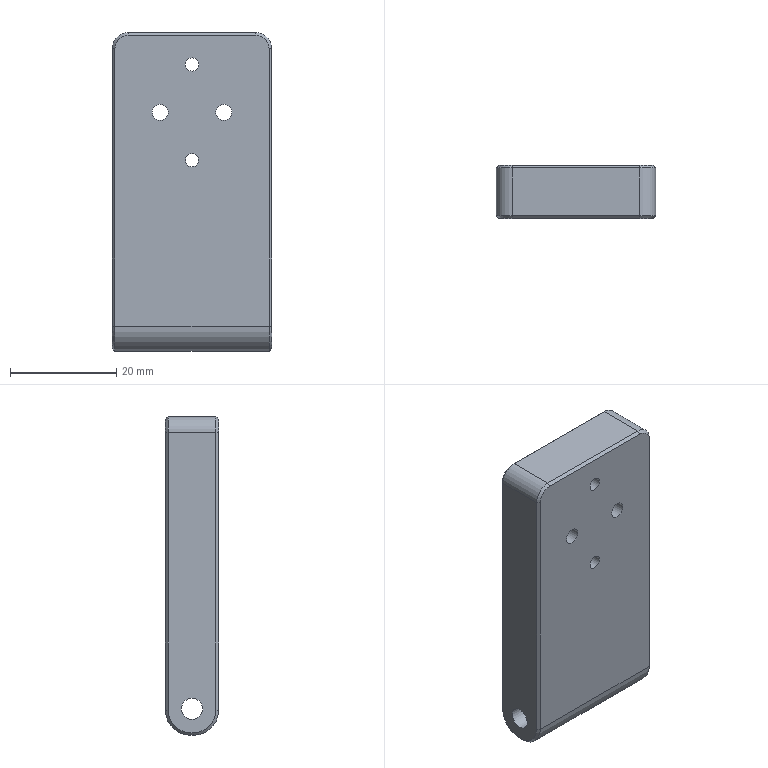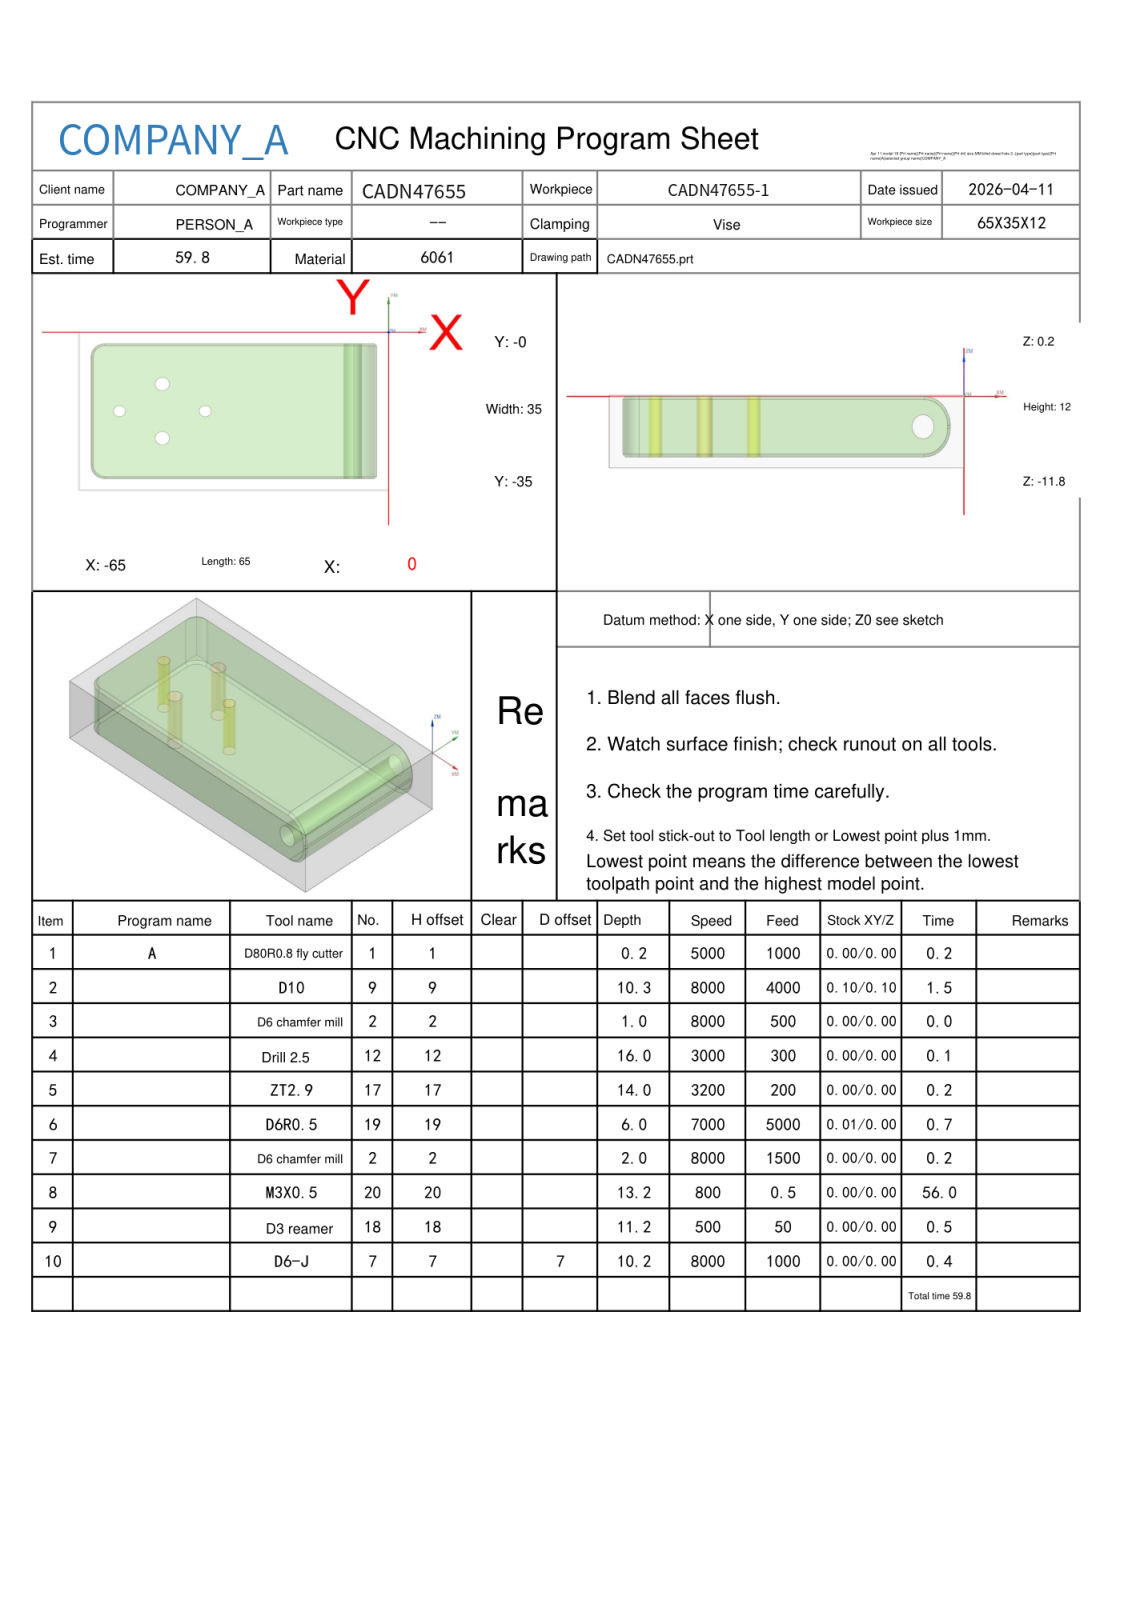NC program | NX | posted by the shop | part box 30 x 10 x 60 mm
Whole program:
%
O0001
(Machine time: 113.76 MIN)
(===Total Tool:9===)
(T1=D80R0.8 fly cutter D=80.  R=0.8  D-  H01 Z=0.    )
(T9=D10     D=10.  R=0.   D-  H09 Z=-10.1 )
(T2=D6 chamfer mill   D=6.   R=0.   D-  H02 Z=-1.8  )
(T12=Drill 2.5  D=2.5  DR_a=118 D-  H12 Z=-15.75)
(T17=ZT2.9  D=2.9  DR_a=120 D-  H17 Z=-13.84)
(T19=D6R0.5 D=6.   R=0.5  D-  H19 Z=-5.75 )
(T20=M3X0.5 D=2.5  DR_a=180 D-  H20 Z=-13.  )
(T18=D3 reamer   D=3.   DR_a=180 D-  H18 Z=-11.  )
(T7=D6-J    D=6.   R=0.   D7  H07 Z=-10.  )
G80 G90 G17 G49 G40
G91 G28 Z0
M01
N1 T01 M06
(D80R0.8 fly cutter  D=80. R=0.8 H=01 ce=0.00 di=0.00)
G00 G90 G54 X-107.5 Y-17.5 M03 S5000
G43 H01 Z20.
M08
Z2.
G01 Z0.0 F1000.
X-102.5
X37.5
X42.5
Z2.
G00 Z20.
G91 G28 Z0.0
M05
M09
G91 G28 Z0.0
M01
N2 T09 M06
(D10  D=10. R=0. H=09 ce=0.10 di=0.10)
G00 G90 G54 X-26.374 Y-47. M03 S8000
G43 H09 Z10.2
M08
Z.761
G01 Z-.439 F4000.
Y-45.979
G03 X-33.374 Y-38.979 I-7. J0.0
G01 X-59.5
G02 X-68.979 Y-29.5 I0.0 J9.479
G01 Y-5.5
G02 X-59.5 Y3.979 I9.479 J0.0
G01 X-7.252
G02 X-2.338 Y2.84 I-.216 J-12.102
X1.372 Y-2.993 I-2.73 J-5.833
G01 Y-32.011
G02 X-2.422 Y-37.887 I-6.447 J0.0
X-7.277 Y-38.979 I-5.086 J11.266
G01 X-33.374
G02 X-33.831 Y-38.617 I0.0 J.47
G01 X-33.893 Y-38.351
G03 X-34.867 Y-37.579 I-.974 J-.228
G01 X-59.5
G02 X-67.579 Y-29.5 I0.0 J8.079
G01 Y-5.5
G02 X-59.5 Y2.579 I8.079 J0.0
G01 X-7.277
G02 X-2.931 Y1.572 I-.191 J-10.702
X-.028 Y-2.993 I-2.137 J-4.565
G01 Y-32.011
G02 X-2.998 Y-36.611 I-5.047 J0.0
X-7.277 Y-37.579 I-4.51 J9.989
G01 X-33.374
X-33.874
G03 X-40.874 Y-44.579 I0.0 J-7.
G01 Y-47.
Z.761
G00 Z3.
G01 X-25.485 F6000.
G00 Z.322
G01 Z-.878 F4000.
Y-46.
G03 X-32.485 Y-39. I-7. J0.0
G01 X-59.5
G02 X-69. Y-29.5 I0.0 J9.5
G01 Y-5.5
G02 X-59.5 Y4. I9.5 J0.0
G01 X-5.472
G02 X-1.822 Y2.954 I-.142 J-7.39
X2.071 Y-3. I-2.716 J-6.026
G01 Y-32.019
G02 X-1.822 Y-37.954 I-6.609 J.091
X-5.498 Y-39. I-3.79 J6.341
G01 X-32.485
G02 X-32.943 Y-38.637 I0.0 J.47
G01 X-33.005 Y-38.372
G03 X-33.978 Y-37.6 I-.974 J-.228
G01 X-59.5
G02 X-67.6 Y-29.5 I0.0 J8.1
G01 Y-5.5
G02 X-59.5 Y2.6 I8.1 J0.0
G01 X-5.499
G02 X-2.471 Y1.711 I-.115 J-5.99
X.671 Y-3. I-2.067 J-4.782
G01 Y-32.
G02 X-2.471 Y-36.711 I-5.209 J.071
X-5.498 Y-37.6 I-3.142 J5.097
G01 X-32.485
X-32.985
G03 X-39.985 Y-44.6 I0.0 J-7.
G01 Y-47.
Z.322
G00 Z2.561
G01 X-25.147 F6000.
G00 Z-.117
G01 Z-1.317 F4000.
Y-44.6
G03 X-32.147 Y-37.6 I-7. J0.0
G01 X-59.5
G02 X-67.6 Y-29.5 I0.0 J8.1
G01 Y-5.5
G02 X-59.5 Y2.6 I8.1 J0.0
G01 X-4.793
G02 X-.945 Y1.1 I-.162 J-6.102
X1.176 Y-3. I-2.947 J-4.123
G01 Y-32.
G02 X-.945 Y-36.1 I-5.068 J.023
X-4.793 Y-37.6 I-4.016 J4.616
G01 X-32.147
X-32.647
G03 X-39.647 Y-44.6 I0.0 J-7.
G01 Y-47.
Z-.117
G00 Z2.122
G01 X-25.147 F6000.
G00 Z-.557
G01 Z-1.757 F4000.
Y-44.6
G03 X-32.147 Y-37.6 I-7. J0.0
G01 X-59.5
G02 X-67.6 Y-29.5 I0.0 J8.1
G01 Y-5.5
G02 X-59.5 Y2.6 I8.1 J0.0
G01 X-4.234
G02 X-.945 Y1.414 I-.045 J-5.278
X1.566 Y-3. I-2.802 J-4.515
G01 Y-32.
G02 X-.945 Y-36.414 I-5.312 J.101
X-4.233 Y-37.6 I-3.326 J4.069
G01 X-32.147
X-32.647
G03 X-39.647 Y-44.6 I0.0 J-7.
G01 Y-47.
Z-.557
G00 Z1.683
G01 X-25.147 F6000.
G00 Z-.996
G01 Z-2.196 F4000.
Y-44.6
G03 X-32.147 Y-37.6 I-7. J0.0
G01 X-59.5
G02 X-67.6 Y-29.5 I0.0 J8.1
G01 Y-5.5
G02 X-59.5 Y2.6 I8.1 J0.0
G01 X-3.896
G02 X-.056 Y.979 I-.053 J-5.486
X1.873 Y-3. I-3.265 J-4.04
G01 Y-32.
G02 X-.056 Y-35.979 I-5.194 J.061
X-3.897 Y-37.6 I-3.911 J3.905
G01 X-32.147
X-32.647
G03 X-39.647 Y-44.6 I0.0 J-7.
G01 Y-47.
Z-.996
G00 Z1.243
G01 X-25.147 F6000.
G00 Z-1.435
G01 Z-2.635 F4000.
Y-44.6
G03 X-32.147 Y-37.6 I-7. J0.0
G01 X-59.5
G02 X-67.6 Y-29.5 I0.0 J8.1
G01 Y-5.5
G02 X-59.5 Y2.6 I8.1 J0.0
G01 X-3.564
G02 X-.056 Y1.213 I-.06 J-5.28
X2.114 Y-3. I-3.244 J-4.337
G01 Y-32.
G02 X-.056 Y-36.213 I-5.415 J.124
X-3.563 Y-37.6 I-3.571 J3.901
G01 X-32.147
X-32.647
G03 X-39.647 Y-44.6 I0.0 J-7.
G01 Y-47.
Z-1.435
G00 Z.804
G01 X-25.147 F6000.
G00 Z-1.874
G01 Z-3.074 F4000.
Y-44.6
G03 X-32.147 Y-37.6 I-7. J0.0
G01 X-59.5
G02 X-67.6 Y-29.5 I0.0 J8.1
G01 Y-5.5
G02 X-59.5 Y2.6 I8.1 J0.0
G01 X-3.345
G02 X.576 Y.817 I-.097 J-5.418
X2.301 Y-3. I-3.456 J-3.86
G01 Y-32.
G02 X.576 Y-35.817 I-5.182 J.043
X-3.345 Y-37.6 I-4.018 J3.634
G01 X-32.147
X-32.647
G03 X-39.647 Y-44.6 I0.0 J-7.
G01 Y-47.
Z-1.874
G00 Z.365
G01 X-25.147 F6000.
G00 Z-2.313
G01 Z-3.513 F4000.
Y-44.6
G03 X-32.147 Y-37.6 I-7. J0.0
G01 X-59.5
G02 X-67.6 Y-29.5 I0.0 J8.1
G01 Y-5.5
G02 X-59.5 Y2.6 I8.1 J0.0
G01 X-3.261
X-3.24
G02 X.701 Y.817 I0.0 J-5.247
X2.44 Y-3. I-3.322 J-3.818
G01 Y-32.
G02 X.701 Y-35.817 I-5.06 J.001
X-3.255 Y-37.6 I-3.956 J3.497
G01 X-3.262
X-32.147
X-32.647
G03 X-39.647 Y-44.6 I0.0 J-7.
G01 Y-47.
Z-2.313
G00 Z-.074
G01 X-25.147 F6000.
G00 Z-2.752
G01 Z-3.952 F4000.
Y-44.6
G03 X-32.147 Y-37.6 I-7. J0.0
G01 X-59.5
G02 X-67.6 Y-29.5 I0.0 J8.1
G01 Y-5.5
G02 X-59.5 Y2.6 I8.1 J0.0
G01 X-3.075
G02 X.558 Y1.054 I-.05 J-5.159
X2.534 Y-3. I-3.379 J-4.156
G01 Y-32.
G02 X.812 Y-35.817 I-5.253 J.073
X-3.075 Y-37.6 I-3.998 J3.588
G01 X-32.147
X-32.647
G03 X-39.647 Y-44.6 I0.0 J-7.
G01 Y-47.
Z-2.752
G00 Z-.513
G01 X-25.147 F6000.
G00 Z-3.191
G01 Z-4.391 F4000.
Y-44.6
G03 X-32.147 Y-37.6 I-7. J0.0
G01 X-59.5
G02 X-67.6 Y-29.5 I0.0 J8.1
G01 Y-5.5
G02 X-59.5 Y2.6 I8.1 J0.0
G01 X-3.015
G02 X.833 Y.849 I-.081 J-5.284
X2.587 Y-3. I-3.579 J-3.955
G01 Y-32.
G02 X.833 Y-35.849 I-5.332 J.105
X-3.015 Y-37.6 I-3.933 J3.542
G01 X-32.147
X-32.647
G03 X-39.647 Y-44.6 I0.0 J-7.
G01 Y-47.
Z-3.191
G00 Z-.952
G01 X-25.147 F6000.
G00 Z-3.63
G01 Z-4.83 F4000.
Y-44.6
G03 X-32.147 Y-37.6 I-7. J0.0
G01 X-59.5
G02 X-67.6 Y-29.5 I0.0 J8.1
G01 Y-5.5
G02 X-59.5 Y2.6 I8.1 J0.0
G01 X-3.015
X-3.
G02 X.606 Y1.106 I0.0 J-5.1
G01 X1.106 Y.606
G02 X2.6 Y-3. I-3.606 J-3.606
G01 Y-32.
G02 X1.106 Y-35.606 I-5.1 J0.0
G01 X.606 Y-36.106
G02 X-3. Y-37.6 I-3.606 J3.606
G01 X-32.147
X-32.647
G03 X-39.647 Y-44.6 I0.0 J-7.
G01 Y-47.
Z-3.63
G00 Z-1.391
G01 X-25.147 F6000.
G00 Z-4.07
G01 Z-5.27 F4000.
Y-44.6
G03 X-32.147 Y-37.6 I-7. J0.0
G01 X-59.5
G02 X-67.6 Y-29.5 I0.0 J8.1
G01 Y-5.5
G02 X-59.5 Y2.6 I8.1 J0.0
G01 X-3.
G02 X.606 Y1.106 I0.0 J-5.1
G01 X1.106 Y.606
G02 X2.6 Y-3. I-3.606 J-3.606
G01 Y-32.
G02 X1.106 Y-35.606 I-5.1 J0.0
G01 X.606 Y-36.106
G02 X-3. Y-37.6 I-3.606 J3.606
G01 X-32.147
X-32.647
G03 X-39.647 Y-44.6 I0.0 J-7.
G01 Y-47.
Z-4.07
G00 Z-1.83
G01 X-25.147 F6000.
G00 Z-4.509
G01 Z-5.709 F4000.
Y-44.6
G03 X-32.147 Y-37.6 I-7. J0.0
G01 X-59.5
G02 X-67.6 Y-29.5 I0.0 J8.1
G01 Y-5.5
G02 X-59.5 Y2.6 I8.1 J0.0
G01 X-3.
G02 X.606 Y1.106 I0.0 J-5.1
G01 X1.106 Y.606
G02 X2.6 Y-3. I-3.606 J-3.606
G01 Y-32.
G02 X1.106 Y-35.606 I-5.1 J0.0
G01 X.606 Y-36.106
G02 X-3. Y-37.6 I-3.606 J3.606
G01 X-32.147
X-32.647
G03 X-39.647 Y-44.6 I0.0 J-7.
G01 Y-47.
Z-4.509
G00 Z-2.27
G01 X-25.147 F6000.
G00 Z-4.948
G01 Z-6.148 F4000.
Y-44.6
G03 X-32.147 Y-37.6 I-7. J0.0
G01 X-59.5
G02 X-67.6 Y-29.5 I0.0 J8.1
G01 Y-5.5
G02 X-59.5 Y2.6 I8.1 J0.0
G01 X-3.
G02 X.606 Y1.106 I0.0 J-5.1
G01 X1.106 Y.606
G02 X2.6 Y-3. I-3.606 J-3.606
G01 Y-32.
G02 X1.106 Y-35.606 I-5.1 J0.0
G01 X.606 Y-36.106
G02 X-3. Y-37.6 I-3.606 J3.606
G01 X-32.147
X-32.647
G03 X-39.647 Y-44.6 I0.0 J-7.
G01 Y-47.
Z-4.948
G00 Z-2.709
G01 X-25.147 F6000.
G00 Z-5.387
G01 Z-6.587 F4000.
Y-44.6
G03 X-32.147 Y-37.6 I-7. J0.0
G01 X-59.5
G02 X-67.6 Y-29.5 I0.0 J8.1
G01 Y-5.5
G02 X-59.5 Y2.6 I8.1 J0.0
G01 X-3.
G02 X.606 Y1.106 I0.0 J-5.1
G01 X1.106 Y.606
G02 X2.6 Y-3. I-3.606 J-3.606
G01 Y-32.
G02 X1.106 Y-35.606 I-5.1 J0.0
G01 X.606 Y-36.106
G02 X-3. Y-37.6 I-3.606 J3.606
G01 X-32.147
X-32.647
G03 X-39.647 Y-44.6 I0.0 J-7.
G01 Y-47.
Z-5.387
G00 Z-3.148
G01 X-25.147 F6000.
G00 Z-5.826
G01 Z-7.026 F4000.
Y-44.6
G03 X-32.147 Y-37.6 I-7. J0.0
G01 X-59.5
G02 X-67.6 Y-29.5 I0.0 J8.1
G01 Y-5.5
G02 X-59.5 Y2.6 I8.1 J0.0
G01 X-3.
G02 X.606 Y1.106 I0.0 J-5.1
G01 X1.106 Y.606
G02 X2.6 Y-3. I-3.606 J-3.606
G01 Y-32.
G02 X1.106 Y-35.606 I-5.1 J0.0
G01 X.606 Y-36.106
G02 X-3. Y-37.6 I-3.606 J3.606
G01 X-32.147
X-32.647
G03 X-39.647 Y-44.6 I0.0 J-7.
G01 Y-47.
Z-5.826
G00 Z-3.587
G01 X-25.147 F6000.
G00 Z-6.265
G01 Z-7.465 F4000.
Y-44.6
G03 X-32.147 Y-37.6 I-7. J0.0
G01 X-59.5
G02 X-67.6 Y-29.5 I0.0 J8.1
G01 Y-5.5
G02 X-59.5 Y2.6 I8.1 J0.0
G01 X-3.
G02 X.606 Y1.106 I0.0 J-5.1
G01 X1.106 Y.606
G02 X2.6 Y-3. I-3.606 J-3.606
G01 Y-32.
G02 X1.106 Y-35.606 I-5.1 J0.0
G01 X.606 Y-36.106
G02 X-3. Y-37.6 I-3.606 J3.606
G01 X-32.147
X-32.647
G03 X-39.647 Y-44.6 I0.0 J-7.
G01 Y-47.
Z-6.265
G00 Z-4.026
G01 X-25.147 F6000.
G00 Z-6.704
G01 Z-7.904 F4000.
Y-44.6
G03 X-32.147 Y-37.6 I-7. J0.0
G01 X-59.5
G02 X-67.6 Y-29.5 I0.0 J8.1
G01 Y-5.5
G02 X-59.5 Y2.6 I8.1 J0.0
G01 X-3.
G02 X.606 Y1.106 I0.0 J-5.1
G01 X1.106 Y.606
G02 X2.6 Y-3. I-3.606 J-3.606
G01 Y-32.
G02 X1.106 Y-35.606 I-5.1 J0.0
G01 X.606 Y-36.106
G02 X-3. Y-37.6 I-3.606 J3.606
G01 X-32.147
X-32.647
G03 X-39.647 Y-44.6 I0.0 J-7.
G01 Y-47.
Z-6.704
G00 Z-4.465
G01 X-25.147 F6000.
G00 Z-7.143
G01 Z-8.343 F4000.
Y-44.6
G03 X-32.147 Y-37.6 I-7. J0.0
G01 X-59.5
G02 X-67.6 Y-29.5 I0.0 J8.1
G01 Y-5.5
G02 X-59.5 Y2.6 I8.1 J0.0
G01 X-3.
G02 X.606 Y1.106 I0.0 J-5.1
G01 X1.106 Y.606
G02 X2.6 Y-3. I-3.606 J-3.606
G01 Y-32.
G02 X1.106 Y-35.606 I-5.1 J0.0
G01 X.606 Y-36.106
G02 X-3. Y-37.6 I-3.606 J3.606
G01 X-32.147
X-32.647
G03 X-39.647 Y-44.6 I0.0 J-7.
G01 Y-47.
Z-7.143
G00 Z-4.904
G01 X-25.147 F6000.
G00 Z-7.583
G01 Z-8.783 F4000.
Y-44.6
G03 X-32.147 Y-37.6 I-7. J0.0
G01 X-59.5
G02 X-67.6 Y-29.5 I0.0 J8.1
G01 Y-5.5
G02 X-59.5 Y2.6 I8.1 J0.0
G01 X-3.
G02 X.606 Y1.106 I0.0 J-5.1
G01 X1.106 Y.606
G02 X2.6 Y-3. I-3.606 J-3.606
G01 Y-32.
G02 X1.106 Y-35.606 I-5.1 J0.0
G01 X.606 Y-36.106
G02 X-3. Y-37.6 I-3.606 J3.606
G01 X-32.147
X-32.647
G03 X-39.647 Y-44.6 I0.0 J-7.
G01 Y-47.
Z-7.583
G00 Z-5.343
G01 X-25.147 F6000.
G00 Z-8.022
G01 Z-9.222 F4000.
Y-44.6
G03 X-32.147 Y-37.6 I-7. J0.0
G01 X-59.5
G02 X-67.6 Y-29.5 I0.0 J8.1
G01 Y-5.5
G02 X-59.5 Y2.6 I8.1 J0.0
G01 X-3.
G02 X.606 Y1.106 I0.0 J-5.1
G01 X1.106 Y.606
G02 X2.6 Y-3. I-3.606 J-3.606
G01 Y-32.
G02 X1.106 Y-35.606 I-5.1 J0.0
G01 X.606 Y-36.106
G02 X-3. Y-37.6 I-3.606 J3.606
G01 X-32.147
X-32.647
G03 X-39.647 Y-44.6 I0.0 J-7.
G01 Y-47.
Z-8.022
G00 Z-5.783
G01 X-25.147 F6000.
G00 Z-8.461
G01 Z-9.661 F4000.
Y-44.6
G03 X-32.147 Y-37.6 I-7. J0.0
G01 X-59.5
G02 X-67.6 Y-29.5 I0.0 J8.1
G01 Y-5.5
G02 X-59.5 Y2.6 I8.1 J0.0
G01 X-3.
G02 X.606 Y1.106 I0.0 J-5.1
G01 X1.106 Y.606
G02 X2.6 Y-3. I-3.606 J-3.606
G01 Y-32.
G02 X1.106 Y-35.606 I-5.1 J0.0
G01 X.606 Y-36.106
G02 X-3. Y-37.6 I-3.606 J3.606
G01 X-32.147
X-32.647
G03 X-39.647 Y-44.6 I0.0 J-7.
G01 Y-47.
Z-8.461
G00 Z-6.222
G01 X-25.147 F6000.
G00 Z-8.9
G01 Z-10.1 F4000.
Y-44.6
G03 X-32.147 Y-37.6 I-7. J0.0
G01 X-59.5
G02 X-67.6 Y-29.5 I0.0 J8.1
G01 Y-5.5
G02 X-59.5 Y2.6 I8.1 J0.0
G01 X-3.
G02 X.606 Y1.106 I0.0 J-5.1
G01 X1.106 Y.606
G02 X2.6 Y-3. I-3.606 J-3.606
G01 Y-32.
G02 X1.106 Y-35.606 I-5.1 J0.0
G01 X.606 Y-36.106
G02 X-3. Y-37.6 I-3.606 J3.606
G01 X-32.147
X-32.647
G03 X-39.647 Y-44.6 I0.0 J-7.
G01 Y-47.
Z-8.9
G00 Z10.2
G91 G28 Z0.0
M05
M09
G91 G28 Z0.0
M01
N3 T02 M06
(D6 chamfer mill  D=6. R=0. H=02 ce=0.00 di=0.10)
G00 G90 G54 X-38.5 Y-17.5 M03 S8000
G43 H02 Z20.
M08
G98 G81 X-38.5 Y-17.5 Z-.8 R1. F500.
X-47.5 Y-23.5
X-56.5 Y-17.5
X-47.5 Y-11.5
G80
G00 Z20.
G91 G28 Z0.0
M05
M09
G91 G28 Z0.0
M01
N4 T12 M06
(Drill 2.5 D=2.5 DR_a=118 H=12)
G00 G90 G54 X-56.5 Y-17.5 M03 S3000
G43 H12 Z20.
M08
G98 G83 X-56.5 Y-17.5 Z-15.751 R1. F300. Q2.
X-38.5
G80
G00 Z20.
G91 G28 Z0.0
M05
M09
G91 G28 Z0.0
M01
N5 T17 M06
(ZT2.9 D=2.9 DR_a=120 H=17)
G00 G90 G54 X-47.5 Y-23.5 M03 S3200
G43 H17 Z20.
M08
G98 G83 X-47.5 Y-23.5 Z-13.837 R1. F200. Q2.
Y-11.5
G80
G00 Z20.
G91 G28 Z0.0
M05
M09
G91 G28 Z0.0
M01
N6 T19 M06
(D6R0.5  D=6. R=0.5 H=19 ce=0.01 di=0.00)
G00 G90 G54 X-11.282 Y2.588 M03 S7000
G43 H19 Z10.2
M08
Z.494
G01 Z-.006 F5000.
Y2.576
G03 X-8.35 Y-.423 I3. J0.0
G02 X-7.836 Y-.406 I.514 J-7.698
X-6.275 Y-.566 I0.0 J-7.715
X-4.486 Y-3. I-.989 J-2.602
G01 Y-32.
G02 X-6.646 Y-34.492 I-2.617 J.086
X-7.832 Y-34.597 I-1.186 J6.688
X-8.35 Y-34.577 I0.0 J6.792
G01 X-8.463 Y-34.622 Z-.013
X-8.349 Y-34.623
X-6.966 Y-34.611
X-6.902 Y-34.605
G03 X-4.367 Y-32. I-.197 J2.728
G01 Y-3.
G03 X-6.902 Y-.395 I-2.734 J-.124
G01 X-6.966 Y-.389
X-8.349 Y-.377
X-8.463 Y-.378
X-8.437 Y-.347 Z-.022
X-6.966 Y-.358
G02 X-4.255 Y-3. I-.039 J-2.753
G01 Y-32.
G02 X-6.713 Y-34.617 I-2.722 J.094
G01 X-6.966 Y-34.642
X-8.437 Y-34.653
X-8.409 Y-34.689 Z-.034
G03 X-7.868 Y-34.703 I.541 J10.769
X-6.551 Y-34.622 I0.0 J10.782
X-4.147 Y-32. I-.335 J2.72
G01 Y-3.
G03 X-6.551 Y-.378 I-2.739 J-.098
X-7.868 Y-.297 I-1.317 J-10.702
X-8.409 Y-.311 I0.0 J-10.782
G01 X-8.388 Y-.284 Z-.047
X-6.966 Y-.291
X-6.62 Y-.323
G02 X-4.042 Y-3. I-.247 J-2.818
G01 Y-32.
G02 X-6.62 Y-34.677 I-2.826 J.142
G01 X-6.966 Y-34.709
X-8.388 Y-34.716
X-8.364 Y-34.747 Z-.062
G03 X-7.783 Y-34.764 I.581 J10.111
X-6.275 Y-34.651 I0.0 J10.127
X-3.939 Y-32. I-.436 J2.739
G01 Y-3.
G03 X-6.275 Y-.349 I-2.772 J-.088
X-7.783 Y-.236 I-1.508 J-10.014
X-8.364 Y-.253 I0.0 J-10.127
G01 X-8.408 Y-.226 Z-.078
G02 X-7.802 Y-.211 I.606 J-11.862
X-6.275 Y-.309 I0.0 J-11.878
X-3.837 Y-3. I-.397 J-2.81
G01 Y-32.
G02 X-6.275 Y-34.691 I-2.835 J.119
X-7.802 Y-34.789 I-1.527 J11.779
X-8.408 Y-34.774 I0.0 J11.878
G01 X-8.387 Y-34.8 Z-.097
X-6.966 Y-34.794
G03 X-5.154 Y-34.336 I-.065 J4.072
X-3.735 Y-32. I-1.213 J2.336
G01 Y-2.948
G03 X-4.214 Y-1.51 I-2.397 J0.0
X-6.62 Y-.227 I-2.574 J-1.93
G01 X-6.966 Y-.206
X-8.387 Y-.2
X-8.364 Y-.171 Z-.118
X-6.966 Y-.184
X-6.62 Y-.203
G02 X-4.191 Y-1.395 I-.111 J-3.299
X-3.635 Y-2.935 I-1.856 J-1.54
G01 Y-32.
G02 X-5.238 Y-34.443 I-2.75 J.056
G01 X-5.432 Y-34.521
G02 X-6.946 Y-34.816 I-1.536 J3.843
G01 X-8.343 Y-34.824
X-8.364 Y-34.829
X-8.361 Y-34.845 Z-.129
X-8.359 Y-34.856 Z-.14
X-6.966 Y-34.841
X-6.955
G03 X-5.238 Y-34.49 I0.0 J4.381
X-3.536 Y-32. I-1.051 J2.545
G01 Y-3.
G03 X-3.855 Y-1.751 I-2.997 J-.1
X-6.275 Y-.214 I-2.728 J-1.621
X-8.051 Y-.142 I-1.776 J-21.903
X-8.359 Y-.144 I0.0 J-21.975
G01 X-8.36 Y-.119 Z-.164
G02 X-7.985 Y-.115 I.375 J-19.937
X-6.275 Y-.189 I0.0 J-19.941
X-3.757 Y-1.761 I-.228 J-3.166
X-3.437 Y-2.949 I-2.047 J-1.189
G01 Y-32.001
G02 X-4.865 Y-34.368 I-2.674 J0.0
X-6.62 Y-34.846 I-1.957 J3.716
G01 X-6.966 Y-34.867
X-8.36 Y-34.881
X-8.351 Y-34.907 Z-.19
G03 X-8.007 Y-34.91 I.343 J27.25
X-6.62 Y-34.874 I0.0 J27.253
X-4.892 Y-34.443 I-.196 J4.465
X-3.339 Y-32. I-1.218 J2.489
G01 Y-3.
G03 X-4.56 Y-.754 I-2.677 J0.0
X-6.275 Y-.161 I-2.055 J-3.169
X-7.895 Y-.087 I-1.62 J-17.514
X-8.351 Y-.093 I0.0 J-17.589
G01 X-8.349 Y-.065 Z-.218
G02 X-7.809 Y-.054 I.54 J-13.475
X-5.929 Y-.186 I0.0 J-13.486
X-3.779 Y-1.408 I-.419 J-3.24
X-3.242 Y-2.962 I-1.979 J-1.554
G01 Y-32.
G02 X-4.892 Y-34.492 I-2.788 J.054
X-6.62 Y-34.904 I-1.964 J4.404
X-7.901 Y-34.94 I-1.281 J22.988
X-8.349 Y-34.935 I0.0 J23.023
G01 Y-34.965 Z-.248
X-6.851 Y-34.951
X-6.62 Y-34.936
G03 X-4.892 Y-34.544 I-.3 J5.335
X-3.146 Y-32. I-1.068 J2.605
G01 Y-2.967
G03 X-3.69 Y-1.397 I-2.535 J0.0
X-5.737 Y-.187 I-2.588 J-2.041
X-7.756 Y-.021 I-2.018 J-12.143
X-8.349 Y-.035 I0.0 J-12.31
G01 Y-.003 Z-.28
G02 X-7.811 Y.004 I.538 J-19.763
X-6.62 Y-.032 I0.0 J-19.771
X-4.892 Y-.4 I-.472 J-6.451
X-3.05 Y-3. I-1.002 J-2.663
G01 Y-32.
G02 X-4.892 Y-34.6 I-2.844 J.063
X-6.966 Y-34.989 I-2.266 J6.353
G01 X-8.349 Y-34.997
Y-35.03 Z-.313
X-7.166 Y-35.023
G03 X-4.884 Y-34.636 I-.041 J7.161
X-2.955 Y-32. I-.927 J2.703
G01 Y-3.
G03 X-4.883 Y-.365 I-2.856 J-.067
X-6.85 Y.014 I-2.317 J-6.745
X-7.812 Y.037 I-.962 J-19.601
X-8.349 Y.03 I0.0 J-19.625
G01 Y.065 Z-.348
G02 X-7.813 Y.073 I.535 J-19.466
X-6.62 Y.036 I0.0 J-19.473
X-4.546 Y-.461 I-.467 J-6.522
X-2.86 Y-3. I-1.152 J-2.594
G01 Y-32.
G02 X-4.546 Y-34.539 I-2.838 J.055
X-7.091 Y-35.058 I-2.585 J6.179
G01 X-8.349 Y-35.065
Y-35.102 Z-.385
X-7.312
X-7.279
G03 X-4.546 Y-34.594 I0.0 J7.605
X-2.767 Y-32. I-1.094 J2.659
G01 Y-3.
G03 X-4.546 Y-.406 I-2.874 J-.064
X-7.163 Y.095 I-2.663 J-6.835
G01 X-8.349 Y.102
Y.141 Z-.424
X-7.236 Y.133
G02 X-4.523 Y-.373 I-.051 J-7.788
X-2.674 Y-3. I-1.018 J-2.681
G01 Y-32.
G02 X-4.546 Y-34.635 I-2.867 J.054
X-7.294 Y-35.141 I-2.748 J7.216
G01 X-7.312
X-8.349
Y-35.181 Z-.464
X-7.312
X-7.304
G03 X-4.546 Y-34.674 I0.0 J7.75
G01 X-4.361 Y-34.605
G03 X-2.582 Y-32. I-1.113 J2.67
G01 Y-3.
G03 X-4.361 Y-.395 I-2.892 J-.065
G01 X-4.546 Y-.326
G03 X-7.182 Y.173 I-2.687 J-6.983
G01 X-8.349 Y.181
Y.223 Z-.506
G02 X-7.819 Y.231 I.53 J-18.812
X-6.823 Y.205 I0.0 J-18.82
X-4.228 Y-.408 I-.396 J-7.479
X-2.49 Y-3. I-1.156 J-2.654
G01 Y-32.
G02 X-4.201 Y-34.58 I-2.894 J.062
X-7.312 Y-35.223 I-3.129 J7.281
G01 X-8.349
Y-35.267 Z-.55
X-7.312
G03 X-4.201 Y-34.627 I-.047 J8.11
X-2.4 Y-32. I-1.101 J2.685
G01 Y-3.
G03 X-4.201 Y-.373 I-2.902 J-.058
X-6.62 Y.236 I-3.222 J-7.689
X-7.82 Y.275 I-1.2 J-18.608
X-8.349 Y.267 I0.0 J-18.646
G01 X-8.341 Y.313 Z-.596
X-6.966 Y.302
G02 X-3.855 Y-.497 I-.304 J-7.64
X-2.311 Y-3. I-1.321 J-2.543
G01 Y-32.
G02 X-3.855 Y-34.503 I-2.866 J.04
X-6.966 Y-35.302 I-3.416 J6.842
G01 X-8.341 Y-35.313
X-8.346 Y-35.36 Z-.643
G03 X-7.923 Y-35.364 I.423 J22.426
X-6.986 Y-35.345 I0.0 J22.43
X-3.852 Y-34.555 I-.332 J7.928
X-2.222 Y-32. I-1.264 J2.604
G01 Y-3.
G03 X-3.852 Y-.445 I-2.894 J-.049
X-6.988 Y.344 I-3.463 J-7.132
X-7.935 Y.364 I-.947 J-22.92
X-8.346 Y.36 I0.0 J-22.939
G01 X-8.341 Y.384 Z-.668
X-8.336 Y.409 Z-.692
G02 X-7.901 Y.414 I.435 J-17.169
X-6.275 Y.337 I0.0 J-17.175
X-3.845 Y-.395 I-1.327 J-8.806
X-2.135 Y-3. I-1.221 J-2.665
G01 Y-32.
G02 X-3.845 Y-34.605 I-2.931 J.06
X-6.62 Y-35.372 I-3.61 J7.658
X-7.917 Y-35.412 I-1.297 J21.012
X-8.336 Y-35.408 I0.0 J21.052
G01 X-8.335 Y-35.433 Z-.717
Y-35.458 Z-.743
X-7.312 Y-35.455
G03 X-3.509 Y-34.473 I-.061 J8.088
X-2.048 Y-32. I-1.428 J2.512
G01 Y-3.
G03 X-3.509 Y-.527 I-2.889 J-.04
X-7.312 Y.454 I-3.858 J-7.093
G01 X-8.334 Y.459
Y.485 Z-.769
X-8.333 Y.511 Z-.795
X-7.312 Y.504
G02 X-3.509 Y-.476 I-.069 J-8.137
X-1.962 Y-3. I-1.352 J-2.565
G01 Y-32.
G02 X-3.509 Y-34.524 I-2.899 J.041
X-7.312 Y-35.505 I-3.88 J7.18
G01 X-8.333 Y-35.51
X-8.332 Y-35.536 Z-.822
X-8.331 Y-35.563 Z-.849
G03 X-7.993 Y-35.565 I.337 J23.996
X-6.966 Y-35.543 I0.0 J23.998
X-3.257 Y-34.426 I-.399 J8.038
X-1.878 Y-32.003 I-1.438 J2.423
G01 Y-2.997
G03 X-3.257 Y-.574 I-2.817 J0.0
X-6.62 Y.517 I-4.1 J-6.907
X-8.034 Y.567 I-1.413 J-20.128
X-8.331 Y.565 I0.0 J-20.177
G01 X-8.329 Y.592 Z-.877
X-8.328 Y.62 Z-.904
G02 X-7.994 Y.624 I.335 J-15.944
X-6.275 Y.531 I0.0 J-15.947
X-3.164 Y-.566 I-1.239 J-8.478
X-1.794 Y-3. I-1.564 J-2.482
G01 Y-32.
G02 X-3.164 Y-34.434 I-2.934 J.048
X-7.312 Y-35.611 I-4.298 J7.251
G01 X-8.328 Y-35.618
X-8.327 Y-35.646 Z-.933
X-8.326 Y-35.674 Z-.961
X-7.312 Y-35.666
G03 X-3.164 Y-34.485 I-.169 J8.468
X-1.712 Y-32. I-1.464 J2.522
G01 Y-3.
G03 X-3.164 Y-.515 I-2.916 J-.038
X-6.275 Y.583 I-4.353 J-7.379
X-8.011 Y.68 I-1.737 J-15.455
X-8.326 Y.677 I0.0 J-15.552
G01 X-8.325 Y.706 Z-.991
X-8.324 Y.735 Z-1.02
G02 X-8.01 Y.738 I.314 J-14.775
X-6.678 Y.678 I0.0 J-14.778
X-2.919 Y-.622 I-.746 J-8.24
X-1.63 Y-2.995 I-1.54 J-2.373
G01 Y-32.001
G02 X-2.934 Y-34.387 I-2.836 J0.0
X-7.312 Y-35.722 I-4.555 J7.093
G01 X-8.324 Y-35.732
X-8.323 Y-35.762 Z-1.05
X-8.322 Y-35.792 Z-1.08
G03 X-8.062 Y-35.794 I.26 J18.062
X-7.015 Y-35.763 I0.0 J18.064
X-2.818 Y-34.373 I-.495 J8.522
X-1.55 Y-32. I-1.656 J2.41
G01 Y-3.
G03 X-2.818 Y-.627 I-2.923 J-.037
X-6.774 Y.745 I-4.685 J-7.118
X-8.015 Y.798 I-1.241 J-14.453
X-8.322 Y.795 I0.0 J-14.506
G01 X-8.321 Y.826 Z-1.111
X-8.32 Y.856 Z-1.142
G02 X-8.091 Y.858 I.229 J-17.323
X-7.016 Y.824 I0.0 J-17.324
X-3.107 Y-.395 I-.534 J-8.591
G01 X-2.818 Y-.565
G02 X-1.471 Y-3. I-1.607 J-2.479
G01 Y-32.
G02 X-2.818 Y-34.435 I-2.957 J.045
G01 X-3.186 Y-34.652
G02 X-7.04 Y-35.824 I-4.34 J7.352
X-8.109 Y-35.854 I-1.07 J18.757
X-8.32 Y-35.853 I0.0 J18.788
G01 X-8.319 Y-35.884 Z-1.173
X-8.317 Y-35.915 Z-1.205
X-8.165 Y-35.916
G03 X-7.064 Y-35.885 I0.0 J19.675
X-3.213 Y-34.717 I-.476 J8.499
G01 X-2.818 Y-34.483
G03 X-1.393 Y-32. I-1.514 J2.519
G01 Y-2.999
G03 X-2.642 Y-.639 I-2.855 J0.0
X-6.275 Y.813 I-5.099 J-7.49
X-8.029 Y.922 I-1.755 J-14.038
X-8.317 Y.919 I0.0 J-14.147
G01 X-8.316 Y.951 Z-1.237
X-8.315 Y.983 Z-1.269
G02 X-8.037 Y.986 I.278 J-13.963
X-6.275 Y.874 I0.0 J-13.966
X-2.543 Y-.651 I-1.543 J-9.1
X-1.317 Y-3. I-1.636 J-2.349
G01 Y-32.003
G02 X-2.538 Y-34.345 I-2.856 J0.0
X-6.275 Y-35.873 I-5.263 J7.538
X-8.06 Y-35.981 I-1.786 J14.652
X-8.315 Y-35.979 I0.0 J14.761
G01 X-8.154 Y-36.042 Z-1.335
X-7.971 Y-36.043
G03 X-6.275 Y-35.936 I0.0 J13.476
X-2.818 Y-34.583 I-1.546 J9.048
G01 X-2.472 Y-34.36
G03 X-1.242 Y-32. I-1.712 J2.394
G01 Y-3.
G03 X-2.472 Y-.64 I-2.943 J-.034
G01 X-2.818 Y-.417
G03 X-6.275 Y.937 I-5.03 J-7.752
X-7.918 Y1.049 I-1.643 J-12.099
X-8.143 Y1.046 I0.0 J-12.21
G01 X-8.024 Y1.068 Z-1.358
X-7.904 Y1.088 Z-1.38
X-7.784 Y1.108 Z-1.403
X-7.599 Y1.11
G02 X-4.736 Y.589 I0.0 J-8.123
G01 X-4.546 Y.517
G02 X-2.349 Y-.678 I-3.452 J-8.965
X-1.168 Y-2.998 I-1.687 J-2.32
G01 Y-32.002
G02 X-2.349 Y-34.322 I-2.868 J0.0
X-5.929 Y-35.939 I-5.687 J7.823
X-7.697 Y-36.101 I-1.768 J9.523
G01 X-7.839 Y-36.1
X-7.682 Y-36.109 Z-1.414
X-7.524 Y-36.117 Z-1.426
X-7.367 Y-36.125 Z-1.437
X-7.209 Y-36.132 Z-1.449
X-7.052 Y-36.133 Z-1.46
X-6.895 Y-36.132 Z-1.472
G03 X-5.238 Y-35.824 I-.404 J6.775
X-2.278 Y-34.328 I-3.116 J9.843
X-1.095 Y-32.004 I-1.691 J2.324
G01 Y-2.998
G03 X-2.272 Y-.676 I-2.879 J0.0
X-4.724 Y.642 I-5.922 J-8.08
X-6.835 Y1.135 I-2.66 J-6.618
G01 X-6.69 Y1.137 Z-1.486
X-6.545 Z-1.5
X-6.4 Y1.132 Z-1.514
X-6.257 Y1.12 Z-1.528
X-6.114 Y1.105 Z-1.542
G02 X-5.002 Y.806 I-.973 J-5.835
G01 X-4.733 Y.705
G02 X-2.108 Y-.74 I-3.708 J-9.845
X-1.023 Y-3. I-1.881 J-2.292
G01 Y-32.
G02 X-2.108 Y-34.26 I-2.965 J.033
X-5.238 Y-35.889 I-6.488 J8.641
X-6.123 Y-36.105 I-1.808 J5.502
G01 X-5.952 Y-36.099 Z-1.566
X-5.781 Y-36.088 Z-1.59
X-5.614 Y-36.064 Z-1.614
G03 X-2.127 Y-34.325 I-2.92 J10.224
X-.953 Y-32. I-1.761 J2.347
G01 Y-3.
G03 X-2.127 Y-.675 I-2.934 J-.022
X-5.613 Y1.064 I-6.428 J-8.522
G01 X-5.487 Y1.052 Z-1.638
X-5.362 Y1.038 Z-1.662
X-5.236 Y1.024 Z-1.686
G02 X-2.022 Y-.699 I-3.738 J-10.831
X-.885 Y-2.999 I-1.755 J-2.299
G01 Y-32.001
G02 X-2.022 Y-34.301 I-2.893 J0.0
X-5.235 Y-36.024 I-6.955 J9.112
G01 X-5.082 Y-36.01 Z-1.723
X-4.932 Y-35.986 Z-1.761
G03 X-2.127 Y-34.43 I-4.357 J11.167
G01 X-1.898 Y-34.26
G03 X-.817 Y-32. I-1.889 J2.291
G01 Y-3.
G03 X-1.898 Y-.74 I-2.969 J-.031
G01 X-2.127 Y-.57
G03 X-4.933 Y.985 I-7.158 J-9.607
G01 X-4.804 Y.968 Z-1.798
X-4.676 Y.949 Z-1.836
G02 X-1.781 Y-.779 I-4.92 J-11.535
X-.752 Y-3. I-1.948 J-2.252
G01 Y-32.
G02 X-1.781 Y-34.221 I-2.977 J.03
X-4.675 Y-35.949 I-7.825 J9.821
G01 X-4.557 Y-35.936 Z-1.874
X-4.443 Y-35.915 Z-1.913
G03 X-1.814 Y-34.305 I-5.913 J12.606
X-.687 Y-32.004 I-1.788 J2.301
G01 Y-2.996
G03 X-1.814 Y-.695 I-2.914 J0.0
X-4.444 Y.915 I-8.53 J-10.979
G01 X-4.339 Y.902 Z-1.952
X-4.237 Y.882 Z-1.991
G02 X-1.691 Y-.74 I-6.428 J-12.895
X-.624 Y-3. I-1.892 J-2.275
G01 Y-32.
G02 X-1.691 Y-34.26 I-2.959 J.015
X-4.236 Y-35.882 I-8.987 J11.289
G01 X-4.14 Y-35.868 Z-2.03
X-4.045 Y-35.849 Z-2.07
G03 X-1.673 Y-34.297 I-7.323 J13.784
X-.563 Y-32.001 I-1.82 J2.296
G01 Y-2.999
G03 X-1.673 Y-.703 I-2.93 J0.0
X-4.046 Y.849 I-9.681 J-12.215
G01 X-3.948 Y.837 Z-2.11
X-3.855 Y.819 Z-2.15
G02 X-2.471 Y-.049 I-18.846 J-31.574
G01 X-1.657 Y-.669
G02 X-.503 Y-2.997 I-1.771 J-2.328
G01 Y-32.003
G02 X-1.657 Y-34.331 I-2.926 J0.0
G01 X-2.471 Y-34.951
G02 X-3.854 Y-35.819 I-19.942 J30.235
G01 X-3.709 Y-35.788 Z-2.231
G03 X-2.928 Y-35.296 I-4.228 J7.582
X-1.435 Y-34.196 I-7.201 J11.33
X-.445 Y-32. I-1.96 J2.206
G01 Y-3.
G03 X-1.435 Y-.804 I-2.951 J-.009
X-2.928 Y.296 I-8.653 J-10.18
X-3.709 Y.788 I-5.02 J-7.107
G01 X-3.558 Y.764 Z-2.314
G02 X-1.435 Y-.747 I-10.232 J-16.617
X-.388 Y-3. I-1.933 J-2.268
G01 Y-32.
G02 X-1.435 Y-34.253 I-2.98 J.016
X-3.558 Y-35.764 I-12.332 J15.073
G01 X-3.422 Y-35.742 Z-2.397
G03 X-1.388 Y-34.26 I-11.283 J17.621
X-.333 Y-32. I-1.928 J2.276
G01 Y-3.
G03 X-1.388 Y-.74 I-2.982 J-.016
X-3.422 Y.742 I-12.952 J-15.643
G01 X-3.294 Y.717 Z-2.482
G02 X-1.332 Y-.74 I-11.6 J-17.664
X-.279 Y-3. I-1.927 J-2.273
G01 Y-32.
G02 X-1.332 Y-34.26 I-2.98 J.014
X-3.294 Y-35.718 I-13.609 J16.259
G01 X-3.164 Y-35.694 Z-2.567
X-2.607 Y-35.296
X-2.472 Y-35.196
X-2.258 Y-35.043
G03 X-1.435 Y-34.387 I-5.978 J8.345
G01 X-1.276 Y-34.26
G03 X-.227 Y-32. I-1.947 J2.277
G01 Y-2.996
G03 X-1.335 Y-.693 I-2.947 J0.0
G01 X-1.435 Y-.613
G03 X-2.26 Y.044 I-6.759 J-7.638
G01 X-2.472 Y.196
X-2.608 Y.296
X-3.165 Y.694
X-3.052 Y.671 Z-2.654
X-3.009 Y.642
X-2.127 Y-.008
X-2.063 Y-.049
G02 X-1.225 Y-.74 I-23.386 J-29.194
X-.177 Y-3. I-1.942 J-2.274
G01 Y-32.
G02 X-1.225 Y-34.26 I-2.991 J.015
X-2.063 Y-34.951 I-24.493 J28.825
G01 X-2.127 Y-34.993
X-3.008 Y-35.642
X-3.052 Y-35.672
X-2.937 Y-35.651 Z-2.741
X-2.004 Y-34.951
X-1.781 Y-34.774
X-1.176 Y-34.26
G03 X-.128 Y-32. I-1.941 J2.272
G01 Y-3.
G03 X-1.176 Y-.74 I-2.988 J-.013
G01 X-1.781 Y-.226
X-2.004 Y-.049
X-2.937 Y.65
X-2.835 Y.631 Z-2.829
X-1.781 Y-.183
X-1.126 Y-.74
G02 X-.081 Y-3. I-1.958 J-2.276
G01 Y-32.
G02 X-1.09 Y-34.226 I-2.991 J.013
G01 X-1.781 Y-34.817
X-1.949 Y-34.951
X-2.127 Y-35.082
X-2.834 Y-35.631
X-2.745 Y-35.616 Z-2.919
X-1.896 Y-34.951
X-1.781 Y-34.86
X-1.09 Y-34.27
G03 X-.036 Y-32. I-1.958 J2.288
G01 Y-3.
G03 X-1.09 Y-.73 I-3.013 J-.019
G01 X-1.781 Y-.14
X-2.746 Y.616
X-2.658 Y.601 Z-3.009
X-2.127 Y.172
X-1.841 Y-.049
G02 X-.903 Y-.868 I-8.475 J-10.66
X.007 Y-2.998 I-2.038 J-2.13
G01 Y-32.
G02 X-.744 Y-33.975 I-3.023 J.02
X-1.841 Y-34.951 I-9.093 J9.119
G01 X-2.127 Y-35.173
X-2.657 Y-35.601
X-2.569 Y-35.584 Z-3.099
X-2.472 Y-35.503
X-1.942 Y-35.076
G03 X-.744 Y-34.023 I-11.432 J14.205
X.049 Y-32. I-2.218 J2.037
G01 Y-2.998
G03 X-.877 Y-.851 I-2.951 J0.0
X-1.927 Y.064 I-12.076 J-12.804
G01 X-2.472 Y.502
X-2.57 Y.584
X-2.484 Y.564 Z-3.191
X-2.127 Y.265
X-1.781 Y-.016
G02 X-.856 Y-.829 I-13.816 J-16.663
X.089 Y-2.999 I-2.018 J-2.171
G01 Y-32.001
G02 X-.857 Y-34.172 I-2.964 J0.0
X-1.781 Y-34.984 I-14.868 J15.992
G01 X-2.127 Y-35.265
X-2.483 Y-35.564
X-2.414 Y-35.553 Z-3.284
G03 X-.744 Y-34.107 I-23.728 J29.093
X.128 Y-32. I-2.164 J2.129
G01 Y-3.
G03 X-.744 Y-.893 I-3.036 J-.023
X-2.415 Y.553 I-25.012 J-27.217
G01 X-2.348 Y.542 Z-3.377
X-1.781 Y.057
X-1.594 Y-.097
G02 X-.65 Y-.956 I-8.265 J-10.027
X.164 Y-3. I-2.2 J-2.061
G01 Y-32.
G02 X-.744 Y-34.144 I-3.038 J.023
G01 X-.872 Y-34.26
X-1.249 Y-34.605
G02 X-1.781 Y-35.058 I-5.654 J6.107
G01 X-2.348 Y-35.543
X-2.281 Y-35.533 Z-3.47
X-1.781 Y-35.095
X-1.606 Y-34.951
G03 X-.83 Y-34.26 I-11.455 J13.643
G01 X-.744 Y-34.178
G03 X.199 Y-32. I-2.11 J2.207
G01 Y-3.
G03 X-.57 Y-1. I-3.063 J-.029
X-1.606 Y-.049 I-10.338 J-10.237
G01 X-1.781 Y.095
X-2.281 Y.532
X-2.217 Y.517 Z-3.565
G02 X-1.781 Y.132 I-26.961 J-30.939
G01 X-1.435 Y-.156
G02 X-.576 Y-.956 I-15.73 J-17.762
X.232 Y-3. I-2.262 J-2.076
G01 Y-32.
G02 X-.576 Y-34.044 I-3.07 J.032
X-1.634 Y-35.01 I-11.465 J11.498
G01 X-1.781 Y-35.132
X-2.217 Y-35.518
X-2.153 Y-35.502 Z-3.66
G03 X-.672 Y-34.173 I-37.004 J42.736
X.263 Y-32. I-2.091 J2.189
G01 Y-3.
G03 X-.545 Y-.956 I-3.026 J-.016
X-1.781 Y.17 I-14.584 J-14.77
X-2.154 Y.501 I-157.33 J-176.326
G01 X-2.102 Y.494 Z-3.755
G02 X-.6 Y-.87 I-31.203 J-35.858
X.293 Y-3. I-2.126 J-2.143
G01 Y-32.
G02 X-.6 Y-34.13 I-3.017 J.013
X-2.101 Y-35.495 I-33.414 J35.249
G01 X-2.058 Y-35.493 Z-3.852
G03 X-.615 Y-34.173 I-50.87 J57.085
X.32 Y-32. I-2.086 J2.186
G01 Y-3.
G03 X-.615 Y-.827 I-3.023 J-.013
X-2.059 Y.493 I-49.787 J-53.041
G01 X-2.02 Y.487 Z-3.948
G02 X-.637 Y-.784 I-37.232 J-41.893
X.346 Y-3. I-2.018 J-2.222
G01 Y-32.
G02 X-.637 Y-34.216 I-3.001 J.005
X-2.019 Y-35.487 I-40.972 J43.154
G01 X-1.98 Y-35.48 Z-4.045
G03 X-.543 Y-34.149 I-32.011 J36.015
X.37 Y-32.001 I-2.072 J2.149
G01 Y-3.
G03 X-.52 Y-.87 I-3.018 J-.01
X-1.981 Y.48 I-34.974 J-36.385
G01 X-1.943 Y.473 Z-4.143
G02 X-.515 Y-.853 I-28.869 J-32.526
X.392 Y-2.998 I-2.083 J-2.145
G01 Y-32.
G02 X-.495 Y-34.13 I-3.034 J.014
X-1.942 Y-35.473 I-34.328 J35.514
G01 X-1.902 Y-35.467 Z-4.241
G03 X-1.435 Y-35.031 I-11.586 J12.886
X-.57 Y-34.216 I-8.24 J9.625
G01 X-.528 Y-34.173
X-.476 Y-34.13
G03 X.412 Y-32. I-2.137 J2.141
G01 Y-2.999
G03 X-.489 Y-.86 I-2.987 J0.0
G01 X-1.09 Y-.274
G02 X-1.904 Y.466 I21.759 J24.734
G01 X-1.867 Y.457 Z-4.339
G02 X-.5 Y-.827 I-51.156 J-55.857
X.43 Y-3. I-2.095 J-2.182
G01 Y-32.
G02 X-.456 Y-34.13 I-3.02 J.007
G01 X-.508 Y-34.173
X-.727 Y-34.392
G02 X-1.435 Y-35.051 I-9.627 J9.637
X-1.865 Y-35.457 I-17.372 J17.922
G01 X-1.829 Y-35.447 Z-4.438
X-1.435 Y-35.071
G03 X-.49 Y-34.173 I-11.902 J13.489
G01 X-.44 Y-34.13
G03 X.447 Y-32. I-2.134 J2.138
G01 Y-3.
G03 X-.484 Y-.827 I-3.025 J-.01
X-1.832 Y.446 I-45.105 J-46.418
G01 X-1.796 Y.435 Z-4.537
X-1.435 Y.09
X-1.09 Y-.225
G02 X-.364 Y-.935 I-9.595 J-10.522
X.461 Y-3. I-2.174 J-2.067
G01 Y-32.
G02 X-.472 Y-34.173 I-3.003 J.002
G01 X-1.09 Y-34.774
G03 X-1.793 Y-35.436 I12.179 J-13.648
G01 X-1.767 Y-35.431 Z-4.636
X-1.435 Y-35.108
G03 X-.413 Y-34.13 I-16.793 J18.574
X.474 Y-32. I-2.115 J2.131
G01 Y-3.
G03 X-.455 Y-.827 I-3.017 J-.005
X-1.77 Y.429 I-50.272 J-51.301
G01 X-1.749 Y.427 Z-4.736
G02 X-.398 Y-.871 I-44.151 J-47.291
X.485 Y-3. I-2.138 J-2.134
G01 Y-32.
G02 X-.398 Y-34.129 I-3.02 J.005
X-1.665 Y-35.347 I-46.758 J47.366
G01 X-1.746 Y-35.43
X-1.727 Y-35.428 Z-4.834
X-1.658 Y-35.354
G03 X-.398 Y-34.135 I-54.504 J57.572
X.493 Y-32. I-2.127 J2.142
G01 Y-3.
G03 X-.437 Y-.827 I-3.023 J-.008
X-1.73 Y.425 I-58.713 J-59.35
G01 X-1.712 Y.421 Z-4.933
G02 X-.343 Y-.913 I-79.65 J-83.045
X.5 Y-3. I-2.188 J-2.098
G01 Y-32.
G02 X-.432 Y-34.173 I-3.031 J.013
X-1.709 Y-35.423 I-244.217 J248.462
G01 X-1.692 Y-35.418 Z-5.032
X-.427 Y-34.173
G03 X.505 Y-32. I-2.093 J2.184
G01 Y-3.
G03 X-.427 Y-.827 I-3.025 J-.011
G01 X-1.667 Y.392
X-1.694 Y.417
X-1.675 Y.413 Z-5.132
X-.335 Y-.913
G02 X.509 Y-3. I-2.163 J-2.089
G01 Y-32.
G02 X-.422 Y-34.173 I-3.008 J.002
G01 X-1.435 Y-35.177
X-1.674 Y-35.413
X-1.657 Y-35.409 Z-5.232
X-1.435 Y-35.189
X-.373 Y-34.13
G03 X.509 Y-32.01 I-2.127 J2.13
G01 Y-2.99
G03 X-.331 Y-.913 I-3.01 J-.01
G01 X-1.658 Y.409
X-1.655 Y.411 Z-5.332
X-.373 Y-.87
G02 X.51 Y-2.99 I-2.128 J-2.13
G01 Y-32.01
G02 X-.373 Y-34.13 I-3.01 J.01
G01 X-1.655 Y-35.411
Z-5.432
X-.373 Y-34.13
G03 X.51 Y-32.01 I-2.127 J2.13
G01 Y-2.99
G03 X-.373 Y-.87 I-3.01 J-.01
G01 X-1.655 Y.411
Z-5.511
X-.373 Y-.87
G02 X.51 Y-2.99 I-2.127 J-2.13
G01 Y-32.01
G02 X-.373 Y-34.13 I-3.01 J.01
G01 X-1.598 Y-35.355
X-1.655 Y-35.411
Z-5.591
X-.373 Y-34.13
G03 X.51 Y-32.01 I-2.127 J2.13
G01 Y-2.99
G03 X-.373 Y-.87 I-3.01 J-.01
G01 X-1.655 Y.411
Z-5.67
X-.331 Y-.913
G02 X.51 Y-2.99 I-2.17 J-2.087
G01 Y-32.01
G02 X-.373 Y-34.13 I-3.01 J.01
G01 X-1.655 Y-35.411
Z-5.75
X-.373 Y-34.13
G03 X.51 Y-32.01 I-2.127 J2.13
G01 Y-2.99
G03 X-.331 Y-.913 I-3.01 J-.01
G01 X-1.655 Y.411
G00 Z10.2
G91 G28 Z0.0
M05
M09
G91 G28 Z0.0
M01
N7 T02 M06
(D6 chamfer mill  D=6. R=0. H=02 ce=0.00 di=0.00)
G00 G90 G54 X-56.5 Y-17.5 M03 S8000
G43 H02 Z20.
M08
G98 G81 X-56.5 Y-17.5 Z-1.75 R3. F500.
X-38.5
G80
G00 Z20.
G00 G90 X-47.5 Y-23.5 M03 S8000
Z20.
G98 G81 X-47.5 Y-23.5 Z-1.8 R3. F500.
Y-11.5
G80
G00 Z20.
G00 G90 X-3.522 Y-33.687 M03 S6500
Z20.
Z.3
G01 Z-1.2 F1500.
G03 X-4.487 Y-33.2 I-.965 J-.713
G01 X-7.03
G03 X-8.23 Y-34.4 I0.0 J-1.2
G01 X-6.05
G03 X-7.25 Y-33.2 I-1.2 J0.0
G01 X-59.5
G02 X-63.2 Y-29.5 I0.0 J3.7
G01 Y-5.5
G02 X-59.5 Y-1.8 I3.7 J0.0
G01 X-4.487
G03 X-3.498 Y-1.28 I0.0 J1.2
G01 Z.3
G00 Z20.
G91 G28 Z0.0
M05
M09
G91 G28 Z0.0
M01
N8 T20 M06
(M3X0.5 D=2.5 DR_a=180 H=20)
G00 G90 G54 X-56.5 Y-17.5 M03 S800
G43 H20 Z20.
M08
G95
G98 G84 X-56.5 Y-17.5 Z-13. R1. F.5 Q5.
X-38.5
G80
G94
G00 Z20.
G91 G28 Z0.0
M05
M09
G91 G28 Z0.0
M01
N9 T18 M06
(D3 reamer D=3. DR_a=180 H=18)
G00 G90 G54 X-47.5 Y-23.5 M03 S500
G43 H18 Z20.
M08
G98 G81 X-47.5 Y-23.5 Z-11. R1. F50.
Y-11.5
G80
G00 Z20.
G91 G28 Z0.0
M05
M09
G91 G28 Z0.0
M01
N10 T07 M06
(D6-J  D=6. R=0. H=07 ce=0.00 di=0.00)
G00 G90 G54 X-60.411 Y1.541 M03 S8000
G43 H07 Z5.2
M08
Z-4.
G01 Z-5. F1000.
G41 D07
X-60.398 Y1.341
G03 X-59.5 Y.5 I.898 J.059
G01 X-3.
G02 X-.879 Y-.379 I0.0 J-3.
G01 X-.379 Y-.879
G02 X.5 Y-3. I-2.121 J-2.121
G01 Y-32.
G02 X-.379 Y-34.121 I-3. J0.0
G01 X-.881 Y-34.623
G02 X-3. Y-35.5 I-2.119 J2.123
G01 X-59.5
G02 X-65.5 Y-29.5 I0.0 J6.
G01 Y-5.5
G02 X-59.5 Y.5 I6. J0.0
G03 X-58.6 Y1.4 I0.0 J.9
G01 G40 Y1.6
Z-4.
G00 X-60.411 Y1.541
Z-9.
G01 Z-10.
G41 D07
X-60.398 Y1.341
G03 X-59.5 Y.5 I.898 J.059
G01 X-3.
G02 X-.879 Y-.379 I0.0 J-3.
G01 X-.379 Y-.879
G02 X.5 Y-3. I-2.121 J-2.121
G01 Y-32.
G02 X-.379 Y-34.121 I-3. J0.0
G01 X-.88 Y-34.622
G02 X-3. Y-35.5 I-2.12 J2.122
G01 X-59.5
G02 X-65.5 Y-29.5 I0.0 J6.
G01 Y-5.5
G02 X-59.5 Y.5 I6. J0.0
G03 X-58.6 Y1.4 I0.0 J.9
G01 G40 Y1.6
Z-9.
G00 Z5.2
M05
M09
G91 G28 Z0.0
G91 G28 Y0.0
M30
%